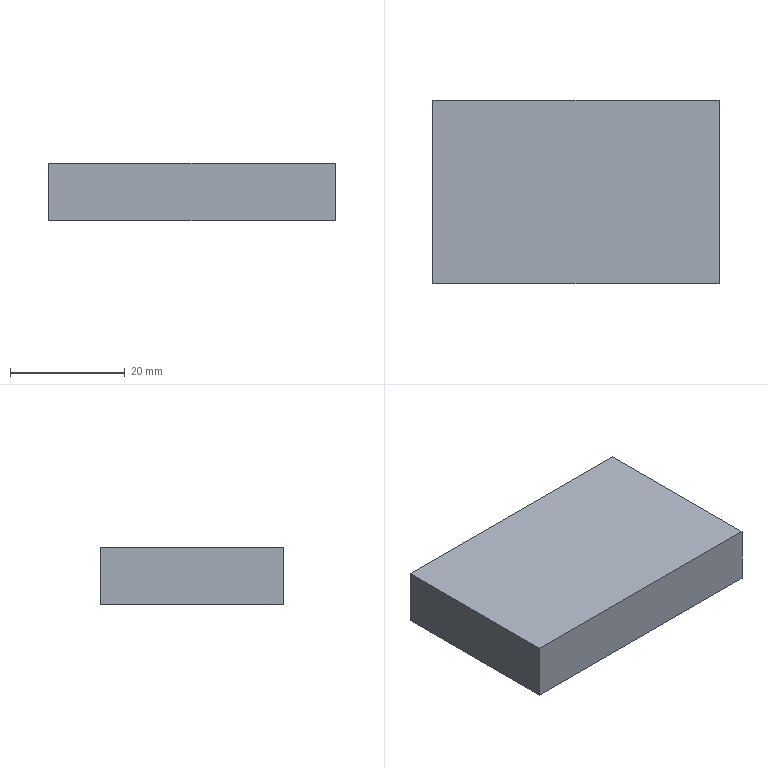Part | NX | features solid 2 | 1 solid | 6 faces | box 50 x 32 x 10 mm | volume 16000 mm3 | plane 6
STEP:
#1=CARTESIAN_POINT('',(-1350.,16.,-670.));
#2=VERTEX_POINT('',#1);
#3=CARTESIAN_POINT('',(-1400.,16.,-670.));
#4=VERTEX_POINT('',#3);
#5=CARTESIAN_POINT('',(-1350.,16.,-670.));
#6=DIRECTION('',(-1.,0.,0.));
#7=VECTOR('',#6,1000.);
#8=LINE('',#5,#7);
#9=EDGE_CURVE('',#2,#4,#8,.T.);
#10=ORIENTED_EDGE('',*,*,#9,.T.);
#11=CARTESIAN_POINT('',(-1400.,16.,-660.));
#12=VERTEX_POINT('',#11);
#13=CARTESIAN_POINT('',(-1400.,16.,-660.));
#14=DIRECTION('',(0.,0.,-1.));
#15=VECTOR('',#14,1000.);
#16=LINE('',#13,#15);
#17=EDGE_CURVE('',#12,#4,#16,.T.);
#18=ORIENTED_EDGE('',*,*,#17,.F.);
#19=CARTESIAN_POINT('',(-1350.,16.,-660.));
#20=VERTEX_POINT('',#19);
#21=CARTESIAN_POINT('',(-1350.,16.,-660.));
#22=DIRECTION('',(-1.,0.,0.));
#23=VECTOR('',#22,1000.);
#24=LINE('',#21,#23);
#25=EDGE_CURVE('',#20,#12,#24,.T.);
#26=ORIENTED_EDGE('',*,*,#25,.F.);
#27=CARTESIAN_POINT('',(-1350.,16.,-660.));
#28=DIRECTION('',(0.,0.,-1.));
#29=VECTOR('',#28,1000.);
#30=LINE('',#27,#29);
#31=EDGE_CURVE('',#20,#2,#30,.T.);
#32=ORIENTED_EDGE('',*,*,#31,.T.);
#33=EDGE_LOOP('',(#10,#18,#26,#32));
#34=FACE_BOUND('',#33,.T.);
#35=CARTESIAN_POINT('',(-1350.,16.,-660.));
#36=DIRECTION('',(0.,-1.,0.));
#37=DIRECTION('',(0.,0.,-1.));
#38=AXIS2_PLACEMENT_3D('',#35,#36,#37);
#39=PLANE('',#38);
#40=ADVANCED_FACE('',(#34),#39,.F.);
#41=CARTESIAN_POINT('',(-1350.,-16.,-670.));
#42=VERTEX_POINT('',#41);
#43=CARTESIAN_POINT('',(-1350.,-50.,-670.));
#44=DIRECTION('',(0.,-1.,0.));
#45=VECTOR('',#44,1000.);
#46=LINE('',#43,#45);
#47=EDGE_CURVE('',#42,#2,#46,.F.);
#48=ORIENTED_EDGE('',*,*,#47,.T.);
#49=ORIENTED_EDGE('',*,*,#31,.F.);
#50=CARTESIAN_POINT('',(-1350.,-16.,-660.));
#51=VERTEX_POINT('',#50);
#52=CARTESIAN_POINT('',(-1350.,-50.,-660.));
#53=DIRECTION('',(0.,-1.,0.));
#54=VECTOR('',#53,1000.);
#55=LINE('',#52,#54);
#56=EDGE_CURVE('',#51,#20,#55,.F.);
#57=ORIENTED_EDGE('',*,*,#56,.F.);
#58=CARTESIAN_POINT('',(-1350.,-16.,-660.));
#59=DIRECTION('',(0.,0.,-1.));
#60=VECTOR('',#59,1000.);
#61=LINE('',#58,#60);
#62=EDGE_CURVE('',#51,#42,#61,.T.);
#63=ORIENTED_EDGE('',*,*,#62,.T.);
#64=EDGE_LOOP('',(#48,#49,#57,#63));
#65=FACE_BOUND('',#64,.T.);
#66=CARTESIAN_POINT('',(-1350.,-50.,-660.));
#67=DIRECTION('',(-1.,0.,0.));
#68=DIRECTION('',(0.,0.,1.));
#69=AXIS2_PLACEMENT_3D('',#66,#67,#68);
#70=PLANE('',#69);
#71=ADVANCED_FACE('',(#65),#70,.F.);
#72=CARTESIAN_POINT('',(-1400.,-16.,-670.));
#73=VERTEX_POINT('',#72);
#74=CARTESIAN_POINT('',(-1350.,-16.,-670.));
#75=DIRECTION('',(1.,0.,0.));
#76=VECTOR('',#75,1000.);
#77=LINE('',#74,#76);
#78=EDGE_CURVE('',#73,#42,#77,.T.);
#79=ORIENTED_EDGE('',*,*,#78,.T.);
#80=ORIENTED_EDGE('',*,*,#62,.F.);
#81=CARTESIAN_POINT('',(-1400.,-16.,-660.));
#82=VERTEX_POINT('',#81);
#83=CARTESIAN_POINT('',(-1350.,-16.,-660.));
#84=DIRECTION('',(1.,0.,0.));
#85=VECTOR('',#84,1000.);
#86=LINE('',#83,#85);
#87=EDGE_CURVE('',#82,#51,#86,.T.);
#88=ORIENTED_EDGE('',*,*,#87,.F.);
#89=CARTESIAN_POINT('',(-1400.,-16.,-660.));
#90=DIRECTION('',(0.,0.,-1.));
#91=VECTOR('',#90,1000.);
#92=LINE('',#89,#91);
#93=EDGE_CURVE('',#82,#73,#92,.T.);
#94=ORIENTED_EDGE('',*,*,#93,.T.);
#95=EDGE_LOOP('',(#79,#80,#88,#94));
#96=FACE_BOUND('',#95,.T.);
#97=CARTESIAN_POINT('',(-1350.,-16.,-660.));
#98=DIRECTION('',(0.,1.,0.));
#99=DIRECTION('',(0.,0.,1.));
#100=AXIS2_PLACEMENT_3D('',#97,#98,#99);
#101=PLANE('',#100);
#102=ADVANCED_FACE('',(#96),#101,.F.);
#103=CARTESIAN_POINT('',(-1400.,-779.99,-670.));
#104=DIRECTION('',(0.,-1.,0.));
#105=VECTOR('',#104,1000.);
#106=LINE('',#103,#105);
#107=EDGE_CURVE('',#4,#73,#106,.T.);
#108=ORIENTED_EDGE('',*,*,#107,.T.);
#109=ORIENTED_EDGE('',*,*,#93,.F.);
#110=CARTESIAN_POINT('',(-1400.,-779.99,-660.));
#111=DIRECTION('',(0.,-1.,0.));
#112=VECTOR('',#111,1000.);
#113=LINE('',#110,#112);
#114=EDGE_CURVE('',#12,#82,#113,.T.);
#115=ORIENTED_EDGE('',*,*,#114,.F.);
#116=ORIENTED_EDGE('',*,*,#17,.T.);
#117=EDGE_LOOP('',(#108,#109,#115,#116));
#118=FACE_BOUND('',#117,.T.);
#119=CARTESIAN_POINT('',(-1400.,-779.99,-660.));
#120=DIRECTION('',(1.,0.,0.));
#121=DIRECTION('',(0.,0.,-1.));
#122=AXIS2_PLACEMENT_3D('',#119,#120,#121);
#123=PLANE('',#122);
#124=ADVANCED_FACE('',(#118),#123,.F.);
#125=ORIENTED_EDGE('',*,*,#25,.T.);
#126=ORIENTED_EDGE('',*,*,#114,.T.);
#127=ORIENTED_EDGE('',*,*,#87,.T.);
#128=ORIENTED_EDGE('',*,*,#56,.T.);
#129=EDGE_LOOP('',(#125,#126,#127,#128));
#130=FACE_BOUND('',#129,.T.);
#131=CARTESIAN_POINT('',(-1350.,0.,-660.));
#132=DIRECTION('',(0.,0.,1.));
#133=DIRECTION('',(-1.,0.,0.));
#134=AXIS2_PLACEMENT_3D('',#131,#132,#133);
#135=PLANE('',#134);
#136=ADVANCED_FACE('',(#130),#135,.T.);
#137=ORIENTED_EDGE('',*,*,#9,.F.);
#138=ORIENTED_EDGE('',*,*,#47,.F.);
#139=ORIENTED_EDGE('',*,*,#78,.F.);
#140=ORIENTED_EDGE('',*,*,#107,.F.);
#141=EDGE_LOOP('',(#137,#138,#139,#140));
#142=FACE_BOUND('',#141,.T.);
#143=CARTESIAN_POINT('',(-1350.,0.,-670.));
#144=DIRECTION('',(0.,0.,1.));
#145=DIRECTION('',(-1.,0.,0.));
#146=AXIS2_PLACEMENT_3D('',#143,#144,#145);
#147=PLANE('',#146);
#148=ADVANCED_FACE('',(#142),#147,.F.);
#149=CLOSED_SHELL('',(#40,#71,#102,#124,#136,#148));
#150=MANIFOLD_SOLID_BREP('',#149);
#151=(LENGTH_UNIT()NAMED_UNIT(*)SI_UNIT(.MILLI.,.METRE.));
#152=UNCERTAINTY_MEASURE_WITH_UNIT(LENGTH_MEASURE(0.00001),#151,'','');
#153=(NAMED_UNIT(*)PLANE_ANGLE_UNIT()SI_UNIT($,.RADIAN.));
#154=(NAMED_UNIT(*)SI_UNIT($,.STERADIAN.)SOLID_ANGLE_UNIT());
#155=(GEOMETRIC_REPRESENTATION_CONTEXT(3)GLOBAL_UNCERTAINTY_ASSIGNED_CONTEXT((#152))GLOBAL_UNIT_ASSIGNED_CONTEXT((#151,#153,#154))REPRESENTATION_CONTEXT('',''));
#156=ADVANCED_BREP_SHAPE_REPRESENTATION('',(#150),#155);